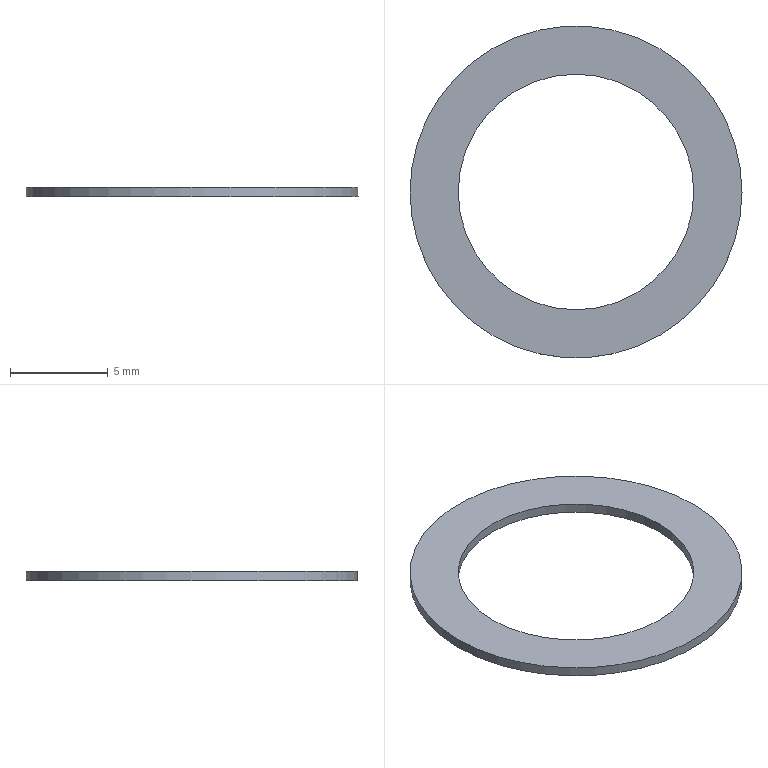Part | NX | features BREP 1 | 1 solid | 4 faces | box 17 x 17 x 0.5 mm | volume 56.374 mm3 | cylinder 2 | plane 2 | commonest cylinder face diameters 12.06 x1 17 x1
STEP:
#1=CARTESIAN_POINT('',(6.03,0.,0.));
#2=VERTEX_POINT('',#1);
#3=CARTESIAN_POINT('',(0.,0.,0.));
#4=DIRECTION('',(0.,0.,1.));
#5=DIRECTION('',(1.,0.,0.));
#6=AXIS2_PLACEMENT_3D('',#3,#4,#5);
#7=CIRCLE('',#6,6.03);
#8=EDGE_CURVE('',#2,#2,#7,.T.);
#9=ORIENTED_EDGE('',*,*,#8,.F.);
#10=EDGE_LOOP('',(#9));
#11=FACE_BOUND('',#10,.T.);
#12=CARTESIAN_POINT('',(6.03,0.,0.5));
#13=VERTEX_POINT('',#12);
#14=CARTESIAN_POINT('',(0.,0.,0.5));
#15=DIRECTION('',(0.,0.,1.));
#16=DIRECTION('',(1.,0.,0.));
#17=AXIS2_PLACEMENT_3D('',#14,#15,#16);
#18=CIRCLE('',#17,6.03);
#19=EDGE_CURVE('',#13,#13,#18,.T.);
#20=ORIENTED_EDGE('',*,*,#19,.T.);
#21=EDGE_LOOP('',(#20));
#22=FACE_BOUND('',#21,.T.);
#23=CARTESIAN_POINT('',(0.,0.,0.5));
#24=DIRECTION('',(0.,0.,-1.));
#25=DIRECTION('',(-1.,0.,0.));
#26=AXIS2_PLACEMENT_3D('',#23,#24,#25);
#27=CYLINDRICAL_SURFACE('',#26,6.03);
#28=ADVANCED_FACE('',(#11,#22),#27,.F.);
#29=CARTESIAN_POINT('',(8.5,0.,0.));
#30=VERTEX_POINT('',#29);
#31=CARTESIAN_POINT('',(0.,0.,0.));
#32=DIRECTION('',(0.,0.,1.));
#33=DIRECTION('',(1.,0.,0.));
#34=AXIS2_PLACEMENT_3D('',#31,#32,#33);
#35=CIRCLE('',#34,8.5);
#36=EDGE_CURVE('',#30,#30,#35,.T.);
#37=ORIENTED_EDGE('',*,*,#36,.T.);
#38=EDGE_LOOP('',(#37));
#39=FACE_BOUND('',#38,.T.);
#40=CARTESIAN_POINT('',(8.5,0.,0.5));
#41=VERTEX_POINT('',#40);
#42=CARTESIAN_POINT('',(0.,0.,0.5));
#43=DIRECTION('',(0.,0.,1.));
#44=DIRECTION('',(1.,0.,0.));
#45=AXIS2_PLACEMENT_3D('',#42,#43,#44);
#46=CIRCLE('',#45,8.5);
#47=EDGE_CURVE('',#41,#41,#46,.T.);
#48=ORIENTED_EDGE('',*,*,#47,.F.);
#49=EDGE_LOOP('',(#48));
#50=FACE_BOUND('',#49,.T.);
#51=CARTESIAN_POINT('',(0.,0.,0.5));
#52=DIRECTION('',(0.,0.,-1.));
#53=DIRECTION('',(-1.,0.,0.));
#54=AXIS2_PLACEMENT_3D('',#51,#52,#53);
#55=CYLINDRICAL_SURFACE('',#54,8.5);
#56=ADVANCED_FACE('',(#39,#50),#55,.T.);
#57=ORIENTED_EDGE('',*,*,#47,.T.);
#58=EDGE_LOOP('',(#57));
#59=FACE_BOUND('',#58,.T.);
#60=ORIENTED_EDGE('',*,*,#19,.F.);
#61=EDGE_LOOP('',(#60));
#62=FACE_BOUND('',#61,.T.);
#63=CARTESIAN_POINT('',(0.,0.,0.5));
#64=DIRECTION('',(0.,0.,1.));
#65=DIRECTION('',(1.,0.,0.));
#66=AXIS2_PLACEMENT_3D('',#63,#64,#65);
#67=PLANE('',#66);
#68=ADVANCED_FACE('',(#59,#62),#67,.T.);
#69=ORIENTED_EDGE('',*,*,#36,.F.);
#70=EDGE_LOOP('',(#69));
#71=FACE_BOUND('',#70,.T.);
#72=ORIENTED_EDGE('',*,*,#8,.T.);
#73=EDGE_LOOP('',(#72));
#74=FACE_BOUND('',#73,.T.);
#75=CARTESIAN_POINT('',(0.,0.,0.));
#76=DIRECTION('',(0.,0.,1.));
#77=DIRECTION('',(1.,0.,0.));
#78=AXIS2_PLACEMENT_3D('',#75,#76,#77);
#79=PLANE('',#78);
#80=ADVANCED_FACE('',(#71,#74),#79,.F.);
#81=CLOSED_SHELL('',(#28,#56,#68,#80));
#82=MANIFOLD_SOLID_BREP('',#81);
#83=(LENGTH_UNIT()NAMED_UNIT(*)SI_UNIT(.MILLI.,.METRE.));
#84=UNCERTAINTY_MEASURE_WITH_UNIT(LENGTH_MEASURE(0.00001),#83,'','');
#85=(NAMED_UNIT(*)PLANE_ANGLE_UNIT()SI_UNIT($,.RADIAN.));
#86=(NAMED_UNIT(*)SI_UNIT($,.STERADIAN.)SOLID_ANGLE_UNIT());
#87=(GEOMETRIC_REPRESENTATION_CONTEXT(3)GLOBAL_UNCERTAINTY_ASSIGNED_CONTEXT((#84))GLOBAL_UNIT_ASSIGNED_CONTEXT((#83,#85,#86))REPRESENTATION_CONTEXT('',''));
#88=ADVANCED_BREP_SHAPE_REPRESENTATION('',(#82),#87);